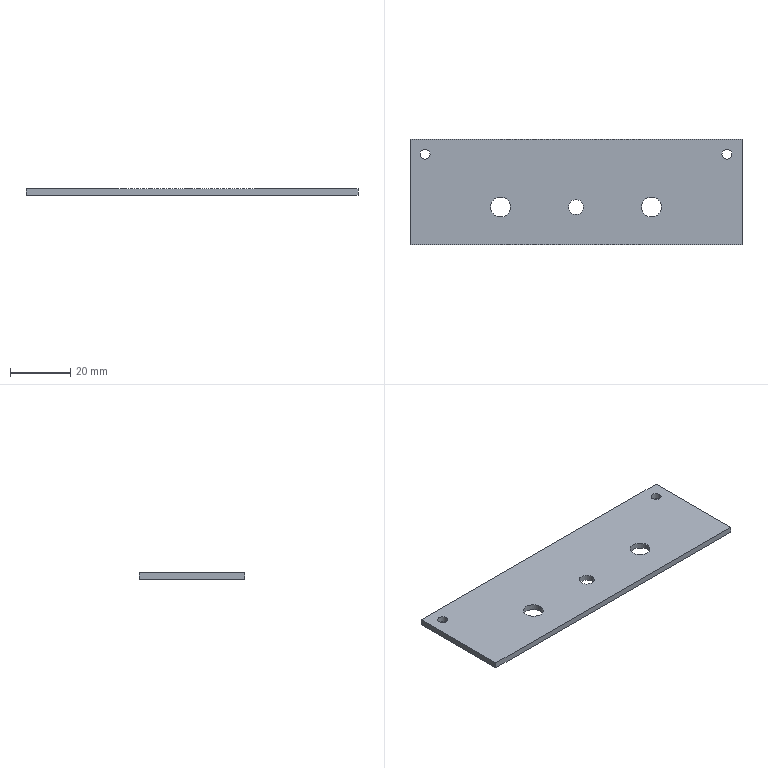Part | SolidWorks | features ICE 3, Extrusion 1 | 1 solid | 16 faces | box 110 x 35 x 2 mm | volume 7490 mm3 | cylinder 10 | plane 6 | commonest cylinder face diameters 3.3 x4 6.6 x4 5 x2
STEP:
#1=CARTESIAN_POINT('',(48.35,17.5,1.));
#2=VERTEX_POINT('',#1);
#3=CARTESIAN_POINT('',(51.65,17.5,1.));
#4=VERTEX_POINT('',#3);
#5=CARTESIAN_POINT('',(50.,17.5,1.));
#6=DIRECTION('',(0.,0.,1.));
#7=DIRECTION('',(1.,0.,0.));
#8=AXIS2_PLACEMENT_3D('',#5,#6,#7);
#9=CIRCLE('',#8,1.65);
#10=EDGE_CURVE('',#2,#4,#9,.T.);
#11=ORIENTED_EDGE('',*,*,#10,.T.);
#12=CARTESIAN_POINT('',(51.65,17.5,-1.));
#13=VERTEX_POINT('',#12);
#14=CARTESIAN_POINT('',(51.65,17.5,9.));
#15=DIRECTION('',(0.,0.,-1.));
#16=VECTOR('',#15,1000.);
#17=LINE('',#14,#16);
#18=EDGE_CURVE('',#4,#13,#17,.T.);
#19=ORIENTED_EDGE('',*,*,#18,.T.);
#20=CARTESIAN_POINT('',(48.35,17.5,-1.));
#21=VERTEX_POINT('',#20);
#22=CARTESIAN_POINT('',(50.,17.5,-1.));
#23=DIRECTION('',(0.,0.,-1.));
#24=DIRECTION('',(-1.,0.,0.));
#25=AXIS2_PLACEMENT_3D('',#22,#23,#24);
#26=CIRCLE('',#25,1.65);
#27=EDGE_CURVE('',#13,#21,#26,.T.);
#28=ORIENTED_EDGE('',*,*,#27,.T.);
#29=CARTESIAN_POINT('',(48.35,17.5,9.));
#30=DIRECTION('',(0.,0.,-1.));
#31=VECTOR('',#30,1000.);
#32=LINE('',#29,#31);
#33=EDGE_CURVE('',#2,#21,#32,.T.);
#34=ORIENTED_EDGE('',*,*,#33,.F.);
#35=EDGE_LOOP('',(#11,#19,#28,#34));
#36=FACE_OUTER_BOUND('',#35,.T.);
#37=CARTESIAN_POINT('',(50.,17.5,9.));
#38=DIRECTION('',(0.,0.,-1.));
#39=DIRECTION('',(-1.,0.,0.));
#40=AXIS2_PLACEMENT_3D('',#37,#38,#39);
#41=CYLINDRICAL_SURFACE('',#40,1.65);
#42=ADVANCED_FACE('',(#36),#41,.F.);
#43=CARTESIAN_POINT('',(-51.65,17.5,1.));
#44=VERTEX_POINT('',#43);
#45=CARTESIAN_POINT('',(-48.35,17.5,1.));
#46=VERTEX_POINT('',#45);
#47=CARTESIAN_POINT('',(-50.,17.5,1.));
#48=DIRECTION('',(0.,0.,1.));
#49=DIRECTION('',(1.,0.,0.));
#50=AXIS2_PLACEMENT_3D('',#47,#48,#49);
#51=CIRCLE('',#50,1.65);
#52=EDGE_CURVE('',#44,#46,#51,.T.);
#53=ORIENTED_EDGE('',*,*,#52,.T.);
#54=CARTESIAN_POINT('',(-48.35,17.5,-1.));
#55=VERTEX_POINT('',#54);
#56=CARTESIAN_POINT('',(-48.35,17.5,9.));
#57=DIRECTION('',(0.,0.,-1.));
#58=VECTOR('',#57,1000.);
#59=LINE('',#56,#58);
#60=EDGE_CURVE('',#46,#55,#59,.T.);
#61=ORIENTED_EDGE('',*,*,#60,.T.);
#62=CARTESIAN_POINT('',(-51.65,17.5,-1.));
#63=VERTEX_POINT('',#62);
#64=CARTESIAN_POINT('',(-50.,17.5,-1.));
#65=DIRECTION('',(0.,0.,-1.));
#66=DIRECTION('',(-1.,0.,0.));
#67=AXIS2_PLACEMENT_3D('',#64,#65,#66);
#68=CIRCLE('',#67,1.65);
#69=EDGE_CURVE('',#55,#63,#68,.T.);
#70=ORIENTED_EDGE('',*,*,#69,.T.);
#71=CARTESIAN_POINT('',(-51.65,17.5,9.));
#72=DIRECTION('',(0.,0.,-1.));
#73=VECTOR('',#72,1000.);
#74=LINE('',#71,#73);
#75=EDGE_CURVE('',#44,#63,#74,.T.);
#76=ORIENTED_EDGE('',*,*,#75,.F.);
#77=EDGE_LOOP('',(#53,#61,#70,#76));
#78=FACE_OUTER_BOUND('',#77,.T.);
#79=CARTESIAN_POINT('',(-50.,17.5,9.));
#80=DIRECTION('',(0.,0.,-1.));
#81=DIRECTION('',(-1.,0.,0.));
#82=AXIS2_PLACEMENT_3D('',#79,#80,#81);
#83=CYLINDRICAL_SURFACE('',#82,1.65);
#84=ADVANCED_FACE('',(#78),#83,.F.);
#85=CARTESIAN_POINT('',(-2.5,0.,-1.));
#86=VERTEX_POINT('',#85);
#87=CARTESIAN_POINT('',(2.5,0.,-1.));
#88=VERTEX_POINT('',#87);
#89=CARTESIAN_POINT('',(0.,0.,-1.));
#90=DIRECTION('',(0.,0.,1.));
#91=DIRECTION('',(1.,0.,0.));
#92=AXIS2_PLACEMENT_3D('',#89,#90,#91);
#93=CIRCLE('',#92,2.5);
#94=EDGE_CURVE('',#86,#88,#93,.T.);
#95=ORIENTED_EDGE('',*,*,#94,.F.);
#96=CARTESIAN_POINT('',(-2.5,0.,1.));
#97=VERTEX_POINT('',#96);
#98=CARTESIAN_POINT('',(-2.5,0.,-9.));
#99=DIRECTION('',(0.,0.,1.));
#100=VECTOR('',#99,1000.);
#101=LINE('',#98,#100);
#102=EDGE_CURVE('',#86,#97,#101,.T.);
#103=ORIENTED_EDGE('',*,*,#102,.T.);
#104=CARTESIAN_POINT('',(2.5,0.,1.));
#105=VERTEX_POINT('',#104);
#106=CARTESIAN_POINT('',(0.,0.,1.));
#107=DIRECTION('',(0.,0.,1.));
#108=DIRECTION('',(1.,0.,0.));
#109=AXIS2_PLACEMENT_3D('',#106,#107,#108);
#110=CIRCLE('',#109,2.5);
#111=EDGE_CURVE('',#97,#105,#110,.T.);
#112=ORIENTED_EDGE('',*,*,#111,.T.);
#113=CARTESIAN_POINT('',(2.5,0.,-9.));
#114=DIRECTION('',(0.,0.,1.));
#115=VECTOR('',#114,1000.);
#116=LINE('',#113,#115);
#117=EDGE_CURVE('',#88,#105,#116,.T.);
#118=ORIENTED_EDGE('',*,*,#117,.F.);
#119=EDGE_LOOP('',(#95,#103,#112,#118));
#120=FACE_OUTER_BOUND('',#119,.T.);
#121=CARTESIAN_POINT('',(0.,0.,-9.));
#122=DIRECTION('',(0.,0.,1.));
#123=DIRECTION('',(1.,0.,0.));
#124=AXIS2_PLACEMENT_3D('',#121,#122,#123);
#125=CYLINDRICAL_SURFACE('',#124,2.5);
#126=ADVANCED_FACE('',(#120),#125,.F.);
#127=CARTESIAN_POINT('',(21.7,0.,1.));
#128=VERTEX_POINT('',#127);
#129=CARTESIAN_POINT('',(28.3,0.,1.));
#130=VERTEX_POINT('',#129);
#131=CARTESIAN_POINT('',(25.,0.,1.));
#132=DIRECTION('',(0.,0.,1.));
#133=DIRECTION('',(1.,0.,0.));
#134=AXIS2_PLACEMENT_3D('',#131,#132,#133);
#135=CIRCLE('',#134,3.3);
#136=EDGE_CURVE('',#128,#130,#135,.T.);
#137=ORIENTED_EDGE('',*,*,#136,.T.);
#138=CARTESIAN_POINT('',(28.3,0.,-1.));
#139=VERTEX_POINT('',#138);
#140=CARTESIAN_POINT('',(28.3,0.,1.));
#141=DIRECTION('',(0.,0.,-1.));
#142=VECTOR('',#141,1000.);
#143=LINE('',#140,#142);
#144=EDGE_CURVE('',#130,#139,#143,.T.);
#145=ORIENTED_EDGE('',*,*,#144,.T.);
#146=CARTESIAN_POINT('',(21.7,0.,-1.));
#147=VERTEX_POINT('',#146);
#148=CARTESIAN_POINT('',(25.,0.,-1.));
#149=DIRECTION('',(0.,0.,1.));
#150=DIRECTION('',(1.,0.,0.));
#151=AXIS2_PLACEMENT_3D('',#148,#149,#150);
#152=CIRCLE('',#151,3.3);
#153=EDGE_CURVE('',#147,#139,#152,.T.);
#154=ORIENTED_EDGE('',*,*,#153,.F.);
#155=CARTESIAN_POINT('',(21.7,0.,1.));
#156=DIRECTION('',(0.,0.,-1.));
#157=VECTOR('',#156,1000.);
#158=LINE('',#155,#157);
#159=EDGE_CURVE('',#128,#147,#158,.T.);
#160=ORIENTED_EDGE('',*,*,#159,.F.);
#161=EDGE_LOOP('',(#137,#145,#154,#160));
#162=FACE_OUTER_BOUND('',#161,.T.);
#163=CARTESIAN_POINT('',(25.,0.,1.));
#164=DIRECTION('',(0.,0.,-1.));
#165=DIRECTION('',(-1.,0.,0.));
#166=AXIS2_PLACEMENT_3D('',#163,#164,#165);
#167=CYLINDRICAL_SURFACE('',#166,3.3);
#168=ADVANCED_FACE('',(#162),#167,.F.);
#169=CARTESIAN_POINT('',(-28.3,0.,1.));
#170=VERTEX_POINT('',#169);
#171=CARTESIAN_POINT('',(-21.7,0.,1.));
#172=VERTEX_POINT('',#171);
#173=CARTESIAN_POINT('',(-25.,0.,1.));
#174=DIRECTION('',(0.,0.,1.));
#175=DIRECTION('',(1.,0.,0.));
#176=AXIS2_PLACEMENT_3D('',#173,#174,#175);
#177=CIRCLE('',#176,3.3);
#178=EDGE_CURVE('',#170,#172,#177,.T.);
#179=ORIENTED_EDGE('',*,*,#178,.T.);
#180=CARTESIAN_POINT('',(-21.7,0.,-1.));
#181=VERTEX_POINT('',#180);
#182=CARTESIAN_POINT('',(-21.7,0.,1.));
#183=DIRECTION('',(0.,0.,-1.));
#184=VECTOR('',#183,1000.);
#185=LINE('',#182,#184);
#186=EDGE_CURVE('',#172,#181,#185,.T.);
#187=ORIENTED_EDGE('',*,*,#186,.T.);
#188=CARTESIAN_POINT('',(-28.3,0.,-1.));
#189=VERTEX_POINT('',#188);
#190=CARTESIAN_POINT('',(-25.,0.,-1.));
#191=DIRECTION('',(0.,0.,1.));
#192=DIRECTION('',(1.,0.,0.));
#193=AXIS2_PLACEMENT_3D('',#190,#191,#192);
#194=CIRCLE('',#193,3.3);
#195=EDGE_CURVE('',#189,#181,#194,.T.);
#196=ORIENTED_EDGE('',*,*,#195,.F.);
#197=CARTESIAN_POINT('',(-28.3,0.,1.));
#198=DIRECTION('',(0.,0.,-1.));
#199=VECTOR('',#198,1000.);
#200=LINE('',#197,#199);
#201=EDGE_CURVE('',#170,#189,#200,.T.);
#202=ORIENTED_EDGE('',*,*,#201,.F.);
#203=EDGE_LOOP('',(#179,#187,#196,#202));
#204=FACE_OUTER_BOUND('',#203,.T.);
#205=CARTESIAN_POINT('',(-25.,0.,1.));
#206=DIRECTION('',(0.,0.,-1.));
#207=DIRECTION('',(-1.,0.,0.));
#208=AXIS2_PLACEMENT_3D('',#205,#206,#207);
#209=CYLINDRICAL_SURFACE('',#208,3.3);
#210=ADVANCED_FACE('',(#204),#209,.F.);
#211=ORIENTED_EDGE('',*,*,#10,.F.);
#212=CARTESIAN_POINT('',(50.,17.5,1.));
#213=DIRECTION('',(0.,0.,1.));
#214=DIRECTION('',(1.,0.,0.));
#215=AXIS2_PLACEMENT_3D('',#212,#213,#214);
#216=CIRCLE('',#215,1.65);
#217=EDGE_CURVE('',#4,#2,#216,.T.);
#218=ORIENTED_EDGE('',*,*,#217,.F.);
#219=EDGE_LOOP('',(#211,#218));
#220=FACE_BOUND('',#219,.T.);
#221=ORIENTED_EDGE('',*,*,#52,.F.);
#222=CARTESIAN_POINT('',(-50.,17.5,1.));
#223=DIRECTION('',(0.,0.,1.));
#224=DIRECTION('',(1.,0.,0.));
#225=AXIS2_PLACEMENT_3D('',#222,#223,#224);
#226=CIRCLE('',#225,1.65);
#227=EDGE_CURVE('',#46,#44,#226,.T.);
#228=ORIENTED_EDGE('',*,*,#227,.F.);
#229=EDGE_LOOP('',(#221,#228));
#230=FACE_BOUND('',#229,.T.);
#231=CARTESIAN_POINT('',(0.,0.,1.));
#232=DIRECTION('',(0.,0.,1.));
#233=DIRECTION('',(1.,0.,0.));
#234=AXIS2_PLACEMENT_3D('',#231,#232,#233);
#235=CIRCLE('',#234,2.5);
#236=EDGE_CURVE('',#105,#97,#235,.T.);
#237=ORIENTED_EDGE('',*,*,#236,.F.);
#238=ORIENTED_EDGE('',*,*,#111,.F.);
#239=EDGE_LOOP('',(#237,#238));
#240=FACE_BOUND('',#239,.T.);
#241=ORIENTED_EDGE('',*,*,#178,.F.);
#242=CARTESIAN_POINT('',(-25.,0.,1.));
#243=DIRECTION('',(0.,0.,1.));
#244=DIRECTION('',(1.,0.,0.));
#245=AXIS2_PLACEMENT_3D('',#242,#243,#244);
#246=CIRCLE('',#245,3.3);
#247=EDGE_CURVE('',#172,#170,#246,.T.);
#248=ORIENTED_EDGE('',*,*,#247,.F.);
#249=EDGE_LOOP('',(#241,#248));
#250=FACE_BOUND('',#249,.T.);
#251=CARTESIAN_POINT('',(-55.,22.5,1.));
#252=VERTEX_POINT('',#251);
#253=CARTESIAN_POINT('',(-55.,-12.5,1.));
#254=VERTEX_POINT('',#253);
#255=CARTESIAN_POINT('',(-55.,-12.5,1.));
#256=DIRECTION('',(0.,-1.,0.));
#257=VECTOR('',#256,1000.);
#258=LINE('',#255,#257);
#259=EDGE_CURVE('',#252,#254,#258,.T.);
#260=ORIENTED_EDGE('',*,*,#259,.T.);
#261=CARTESIAN_POINT('',(55.,-12.5,1.));
#262=VERTEX_POINT('',#261);
#263=CARTESIAN_POINT('',(55.,-12.5,1.));
#264=DIRECTION('',(1.,0.,0.));
#265=VECTOR('',#264,1000.);
#266=LINE('',#263,#265);
#267=EDGE_CURVE('',#254,#262,#266,.T.);
#268=ORIENTED_EDGE('',*,*,#267,.T.);
#269=CARTESIAN_POINT('',(55.,22.5,1.));
#270=VERTEX_POINT('',#269);
#271=CARTESIAN_POINT('',(55.,-12.5,1.));
#272=DIRECTION('',(0.,1.,0.));
#273=VECTOR('',#272,1000.);
#274=LINE('',#271,#273);
#275=EDGE_CURVE('',#262,#270,#274,.T.);
#276=ORIENTED_EDGE('',*,*,#275,.T.);
#277=CARTESIAN_POINT('',(-55.,22.5,1.));
#278=DIRECTION('',(1.,0.,0.));
#279=VECTOR('',#278,1000.);
#280=LINE('',#277,#279);
#281=EDGE_CURVE('',#252,#270,#280,.T.);
#282=ORIENTED_EDGE('',*,*,#281,.F.);
#283=EDGE_LOOP('',(#260,#268,#276,#282));
#284=FACE_OUTER_BOUND('',#283,.T.);
#285=ORIENTED_EDGE('',*,*,#136,.F.);
#286=CARTESIAN_POINT('',(25.,0.,1.));
#287=DIRECTION('',(0.,0.,1.));
#288=DIRECTION('',(1.,0.,0.));
#289=AXIS2_PLACEMENT_3D('',#286,#287,#288);
#290=CIRCLE('',#289,3.3);
#291=EDGE_CURVE('',#130,#128,#290,.T.);
#292=ORIENTED_EDGE('',*,*,#291,.F.);
#293=EDGE_LOOP('',(#285,#292));
#294=FACE_BOUND('',#293,.T.);
#295=CARTESIAN_POINT('',(0.,0.,1.));
#296=DIRECTION('',(0.,0.,1.));
#297=DIRECTION('',(1.,0.,0.));
#298=AXIS2_PLACEMENT_3D('',#295,#296,#297);
#299=PLANE('',#298);
#300=ADVANCED_FACE('',(#220,#230,#240,#250,#284,#294),#299,.T.);
#301=CARTESIAN_POINT('',(50.,17.5,-1.));
#302=DIRECTION('',(0.,0.,-1.));
#303=DIRECTION('',(-1.,0.,0.));
#304=AXIS2_PLACEMENT_3D('',#301,#302,#303);
#305=CIRCLE('',#304,1.65);
#306=EDGE_CURVE('',#21,#13,#305,.T.);
#307=ORIENTED_EDGE('',*,*,#306,.F.);
#308=ORIENTED_EDGE('',*,*,#27,.F.);
#309=EDGE_LOOP('',(#307,#308));
#310=FACE_BOUND('',#309,.T.);
#311=CARTESIAN_POINT('',(-50.,17.5,-1.));
#312=DIRECTION('',(0.,0.,-1.));
#313=DIRECTION('',(-1.,0.,0.));
#314=AXIS2_PLACEMENT_3D('',#311,#312,#313);
#315=CIRCLE('',#314,1.65);
#316=EDGE_CURVE('',#63,#55,#315,.T.);
#317=ORIENTED_EDGE('',*,*,#316,.F.);
#318=ORIENTED_EDGE('',*,*,#69,.F.);
#319=EDGE_LOOP('',(#317,#318));
#320=FACE_BOUND('',#319,.T.);
#321=CARTESIAN_POINT('',(0.,0.,-1.));
#322=DIRECTION('',(0.,0.,1.));
#323=DIRECTION('',(1.,0.,0.));
#324=AXIS2_PLACEMENT_3D('',#321,#322,#323);
#325=CIRCLE('',#324,2.5);
#326=EDGE_CURVE('',#88,#86,#325,.T.);
#327=ORIENTED_EDGE('',*,*,#326,.T.);
#328=ORIENTED_EDGE('',*,*,#94,.T.);
#329=EDGE_LOOP('',(#327,#328));
#330=FACE_BOUND('',#329,.T.);
#331=CARTESIAN_POINT('',(-55.,22.5,-1.));
#332=VERTEX_POINT('',#331);
#333=CARTESIAN_POINT('',(-55.,-12.5,-1.));
#334=VERTEX_POINT('',#333);
#335=CARTESIAN_POINT('',(-55.,-12.5,-1.));
#336=DIRECTION('',(0.,-1.,0.));
#337=VECTOR('',#336,1000.);
#338=LINE('',#335,#337);
#339=EDGE_CURVE('',#332,#334,#338,.T.);
#340=ORIENTED_EDGE('',*,*,#339,.F.);
#341=CARTESIAN_POINT('',(55.,22.5,-1.));
#342=VERTEX_POINT('',#341);
#343=CARTESIAN_POINT('',(55.,22.5,-1.));
#344=DIRECTION('',(-1.,0.,0.));
#345=VECTOR('',#344,1000.);
#346=LINE('',#343,#345);
#347=EDGE_CURVE('',#342,#332,#346,.T.);
#348=ORIENTED_EDGE('',*,*,#347,.F.);
#349=CARTESIAN_POINT('',(55.,-12.5,-1.));
#350=VERTEX_POINT('',#349);
#351=CARTESIAN_POINT('',(55.,-12.5,-1.));
#352=DIRECTION('',(0.,1.,0.));
#353=VECTOR('',#352,1000.);
#354=LINE('',#351,#353);
#355=EDGE_CURVE('',#350,#342,#354,.T.);
#356=ORIENTED_EDGE('',*,*,#355,.F.);
#357=CARTESIAN_POINT('',(55.,-12.5,-1.));
#358=DIRECTION('',(1.,0.,0.));
#359=VECTOR('',#358,1000.);
#360=LINE('',#357,#359);
#361=EDGE_CURVE('',#334,#350,#360,.T.);
#362=ORIENTED_EDGE('',*,*,#361,.F.);
#363=EDGE_LOOP('',(#340,#348,#356,#362));
#364=FACE_OUTER_BOUND('',#363,.T.);
#365=ORIENTED_EDGE('',*,*,#195,.T.);
#366=CARTESIAN_POINT('',(-25.,0.,-1.));
#367=DIRECTION('',(0.,0.,1.));
#368=DIRECTION('',(1.,0.,0.));
#369=AXIS2_PLACEMENT_3D('',#366,#367,#368);
#370=CIRCLE('',#369,3.3);
#371=EDGE_CURVE('',#181,#189,#370,.T.);
#372=ORIENTED_EDGE('',*,*,#371,.T.);
#373=EDGE_LOOP('',(#365,#372));
#374=FACE_BOUND('',#373,.T.);
#375=ORIENTED_EDGE('',*,*,#153,.T.);
#376=CARTESIAN_POINT('',(25.,0.,-1.));
#377=DIRECTION('',(0.,0.,1.));
#378=DIRECTION('',(1.,0.,0.));
#379=AXIS2_PLACEMENT_3D('',#376,#377,#378);
#380=CIRCLE('',#379,3.3);
#381=EDGE_CURVE('',#139,#147,#380,.T.);
#382=ORIENTED_EDGE('',*,*,#381,.T.);
#383=EDGE_LOOP('',(#375,#382));
#384=FACE_BOUND('',#383,.T.);
#385=CARTESIAN_POINT('',(0.,0.,-1.));
#386=DIRECTION('',(0.,0.,1.));
#387=DIRECTION('',(1.,0.,0.));
#388=AXIS2_PLACEMENT_3D('',#385,#386,#387);
#389=PLANE('',#388);
#390=ADVANCED_FACE('',(#310,#320,#330,#364,#374,#384),#389,.F.);
#391=ORIENTED_EDGE('',*,*,#339,.T.);
#392=CARTESIAN_POINT('',(-55.,-12.5,1.));
#393=DIRECTION('',(0.,0.,-1.));
#394=VECTOR('',#393,1000.);
#395=LINE('',#392,#394);
#396=EDGE_CURVE('',#254,#334,#395,.T.);
#397=ORIENTED_EDGE('',*,*,#396,.F.);
#398=ORIENTED_EDGE('',*,*,#259,.F.);
#399=CARTESIAN_POINT('',(-55.,22.5,-1.));
#400=DIRECTION('',(0.,0.,1.));
#401=VECTOR('',#400,1000.);
#402=LINE('',#399,#401);
#403=EDGE_CURVE('',#332,#252,#402,.T.);
#404=ORIENTED_EDGE('',*,*,#403,.F.);
#405=EDGE_LOOP('',(#391,#397,#398,#404));
#406=FACE_OUTER_BOUND('',#405,.T.);
#407=CARTESIAN_POINT('',(-55.,-12.5,1.));
#408=DIRECTION('',(1.,0.,0.));
#409=DIRECTION('',(0.,0.,-1.));
#410=AXIS2_PLACEMENT_3D('',#407,#408,#409);
#411=PLANE('',#410);
#412=ADVANCED_FACE('',(#406),#411,.F.);
#413=ORIENTED_EDGE('',*,*,#361,.T.);
#414=CARTESIAN_POINT('',(55.,-12.5,1.));
#415=DIRECTION('',(0.,0.,-1.));
#416=VECTOR('',#415,1000.);
#417=LINE('',#414,#416);
#418=EDGE_CURVE('',#262,#350,#417,.T.);
#419=ORIENTED_EDGE('',*,*,#418,.F.);
#420=ORIENTED_EDGE('',*,*,#267,.F.);
#421=ORIENTED_EDGE('',*,*,#396,.T.);
#422=EDGE_LOOP('',(#413,#419,#420,#421));
#423=FACE_OUTER_BOUND('',#422,.T.);
#424=CARTESIAN_POINT('',(55.,-12.5,1.));
#425=DIRECTION('',(0.,1.,0.));
#426=DIRECTION('',(-1.,0.,0.));
#427=AXIS2_PLACEMENT_3D('',#424,#425,#426);
#428=PLANE('',#427);
#429=ADVANCED_FACE('',(#423),#428,.F.);
#430=ORIENTED_EDGE('',*,*,#355,.T.);
#431=CARTESIAN_POINT('',(55.,22.5,1.));
#432=DIRECTION('',(0.,0.,-1.));
#433=VECTOR('',#432,1000.);
#434=LINE('',#431,#433);
#435=EDGE_CURVE('',#270,#342,#434,.T.);
#436=ORIENTED_EDGE('',*,*,#435,.F.);
#437=ORIENTED_EDGE('',*,*,#275,.F.);
#438=ORIENTED_EDGE('',*,*,#418,.T.);
#439=EDGE_LOOP('',(#430,#436,#437,#438));
#440=FACE_OUTER_BOUND('',#439,.T.);
#441=CARTESIAN_POINT('',(55.,-12.5,1.));
#442=DIRECTION('',(-1.,0.,0.));
#443=DIRECTION('',(0.,0.,1.));
#444=AXIS2_PLACEMENT_3D('',#441,#442,#443);
#445=PLANE('',#444);
#446=ADVANCED_FACE('',(#440),#445,.F.);
#447=ORIENTED_EDGE('',*,*,#186,.F.);
#448=ORIENTED_EDGE('',*,*,#247,.T.);
#449=ORIENTED_EDGE('',*,*,#201,.T.);
#450=ORIENTED_EDGE('',*,*,#371,.F.);
#451=EDGE_LOOP('',(#447,#448,#449,#450));
#452=FACE_OUTER_BOUND('',#451,.T.);
#453=CARTESIAN_POINT('',(-25.,0.,1.));
#454=DIRECTION('',(0.,0.,-1.));
#455=DIRECTION('',(-1.,0.,0.));
#456=AXIS2_PLACEMENT_3D('',#453,#454,#455);
#457=CYLINDRICAL_SURFACE('',#456,3.3);
#458=ADVANCED_FACE('',(#452),#457,.F.);
#459=ORIENTED_EDGE('',*,*,#144,.F.);
#460=ORIENTED_EDGE('',*,*,#291,.T.);
#461=ORIENTED_EDGE('',*,*,#159,.T.);
#462=ORIENTED_EDGE('',*,*,#381,.F.);
#463=EDGE_LOOP('',(#459,#460,#461,#462));
#464=FACE_OUTER_BOUND('',#463,.T.);
#465=CARTESIAN_POINT('',(25.,0.,1.));
#466=DIRECTION('',(0.,0.,-1.));
#467=DIRECTION('',(-1.,0.,0.));
#468=AXIS2_PLACEMENT_3D('',#465,#466,#467);
#469=CYLINDRICAL_SURFACE('',#468,3.3);
#470=ADVANCED_FACE('',(#464),#469,.F.);
#471=ORIENTED_EDGE('',*,*,#102,.F.);
#472=ORIENTED_EDGE('',*,*,#326,.F.);
#473=ORIENTED_EDGE('',*,*,#117,.T.);
#474=ORIENTED_EDGE('',*,*,#236,.T.);
#475=EDGE_LOOP('',(#471,#472,#473,#474));
#476=FACE_OUTER_BOUND('',#475,.T.);
#477=CARTESIAN_POINT('',(0.,0.,-9.));
#478=DIRECTION('',(0.,0.,1.));
#479=DIRECTION('',(1.,0.,0.));
#480=AXIS2_PLACEMENT_3D('',#477,#478,#479);
#481=CYLINDRICAL_SURFACE('',#480,2.5);
#482=ADVANCED_FACE('',(#476),#481,.F.);
#483=ORIENTED_EDGE('',*,*,#435,.T.);
#484=ORIENTED_EDGE('',*,*,#347,.T.);
#485=ORIENTED_EDGE('',*,*,#403,.T.);
#486=ORIENTED_EDGE('',*,*,#281,.T.);
#487=EDGE_LOOP('',(#483,#484,#485,#486));
#488=FACE_OUTER_BOUND('',#487,.T.);
#489=CARTESIAN_POINT('',(0.,22.5,0.));
#490=DIRECTION('',(0.,1.,0.));
#491=DIRECTION('',(-1.,0.,0.));
#492=AXIS2_PLACEMENT_3D('',#489,#490,#491);
#493=PLANE('',#492);
#494=ADVANCED_FACE('',(#488),#493,.T.);
#495=ORIENTED_EDGE('',*,*,#60,.F.);
#496=ORIENTED_EDGE('',*,*,#227,.T.);
#497=ORIENTED_EDGE('',*,*,#75,.T.);
#498=ORIENTED_EDGE('',*,*,#316,.T.);
#499=EDGE_LOOP('',(#495,#496,#497,#498));
#500=FACE_OUTER_BOUND('',#499,.T.);
#501=CARTESIAN_POINT('',(-50.,17.5,9.));
#502=DIRECTION('',(0.,0.,-1.));
#503=DIRECTION('',(-1.,0.,0.));
#504=AXIS2_PLACEMENT_3D('',#501,#502,#503);
#505=CYLINDRICAL_SURFACE('',#504,1.65);
#506=ADVANCED_FACE('',(#500),#505,.F.);
#507=ORIENTED_EDGE('',*,*,#18,.F.);
#508=ORIENTED_EDGE('',*,*,#217,.T.);
#509=ORIENTED_EDGE('',*,*,#33,.T.);
#510=ORIENTED_EDGE('',*,*,#306,.T.);
#511=EDGE_LOOP('',(#507,#508,#509,#510));
#512=FACE_OUTER_BOUND('',#511,.T.);
#513=CARTESIAN_POINT('',(50.,17.5,9.));
#514=DIRECTION('',(0.,0.,-1.));
#515=DIRECTION('',(-1.,0.,0.));
#516=AXIS2_PLACEMENT_3D('',#513,#514,#515);
#517=CYLINDRICAL_SURFACE('',#516,1.65);
#518=ADVANCED_FACE('',(#512),#517,.F.);
#519=CLOSED_SHELL('',(#42,#84,#126,#168,#210,#300,#390,#412,#429,#446,#458,#470,#482,#494,#506,#518));
#520=MANIFOLD_SOLID_BREP('',#519);
#521=CARTESIAN_POINT('',(0.,0.,0.));
#522=DIRECTION('',(0.,0.,1.));
#523=DIRECTION('',(1.,0.,0.));
#524=AXIS2_PLACEMENT_3D('',#521,#522,#523);
#525=(LENGTH_UNIT()NAMED_UNIT(*)SI_UNIT(.MILLI.,.METRE.));
#526=UNCERTAINTY_MEASURE_WITH_UNIT(LENGTH_MEASURE(0.00001),#525,'','');
#527=(NAMED_UNIT(*)PLANE_ANGLE_UNIT()SI_UNIT($,.RADIAN.));
#528=(NAMED_UNIT(*)SI_UNIT($,.STERADIAN.)SOLID_ANGLE_UNIT());
#529=(GEOMETRIC_REPRESENTATION_CONTEXT(3)GLOBAL_UNCERTAINTY_ASSIGNED_CONTEXT((#526))GLOBAL_UNIT_ASSIGNED_CONTEXT((#525,#527,#528))REPRESENTATION_CONTEXT('',''));
#530=ADVANCED_BREP_SHAPE_REPRESENTATION('',(#520,#524),#529);